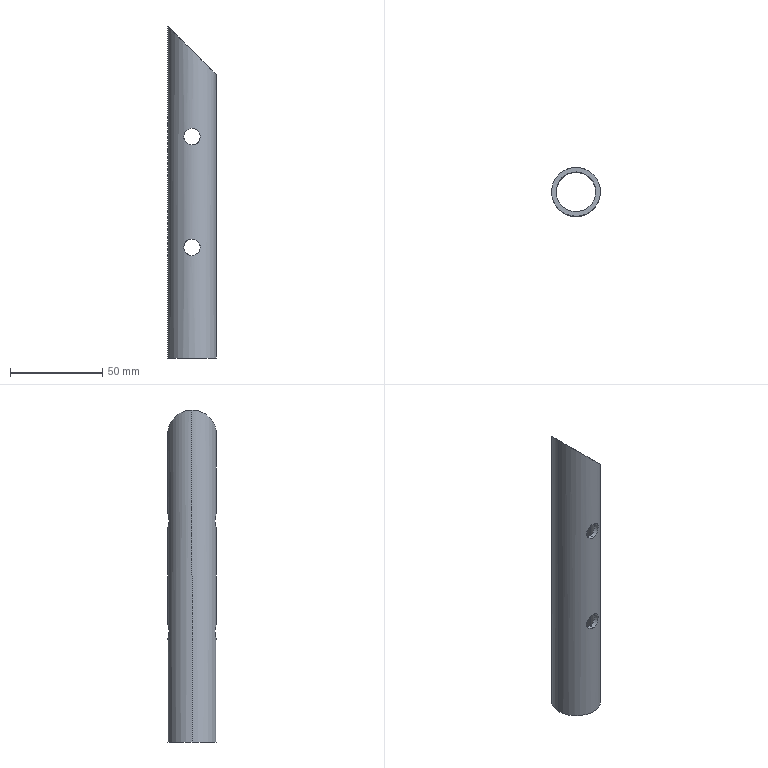Part | NX | features BREP 1 | 1 solid | 14 faces | box 26.5 x 26.5 x 180 mm | volume 30784 mm3 | cylinder 12 | plane 2 | commonest cylinder face diameters 9 x8 21.5 x2 26.5 x2
STEP:
#1=CARTESIAN_POINT('',(0.,10.75,25.5));
#2=VERTEX_POINT('',#1);
#3=CARTESIAN_POINT('',(0.,10.75,34.5));
#4=VERTEX_POINT('',#3);
#5=CARTESIAN_POINT('',(0.,10.75,25.5));
#6=CARTESIAN_POINT('',(1.204,10.75,25.5));
#7=CARTESIAN_POINT('',(3.514,10.279,26.479));
#8=CARTESIAN_POINT('',(4.992,9.505,29.99));
#9=CARTESIAN_POINT('',(3.516,10.279,33.525));
#10=CARTESIAN_POINT('',(1.204,10.75,34.5));
#11=CARTESIAN_POINT('',(0.,10.75,34.5));
#12=B_SPLINE_CURVE_WITH_KNOTS('',3,(#5,#6,#7,#8,#9,#10,#11),.UNSPECIFIED.,.F.,.F.,(4,1,1,1,4),(0.,0.003557,0.007114,0.01067,0.01423),.UNSPECIFIED.);
#13=EDGE_CURVE('',#2,#4,#12,.T.);
#14=ORIENTED_EDGE('',*,*,#13,.T.);
#15=CARTESIAN_POINT('',(0.,13.25,34.5));
#16=VERTEX_POINT('',#15);
#17=CARTESIAN_POINT('',(0.,13.25,34.5));
#18=DIRECTION('',(0.,-1.,0.));
#19=VECTOR('',#18,1000.);
#20=LINE('',#17,#19);
#21=EDGE_CURVE('',#16,#4,#20,.T.);
#22=ORIENTED_EDGE('',*,*,#21,.F.);
#23=CARTESIAN_POINT('',(0.,13.25,25.5));
#24=VERTEX_POINT('',#23);
#25=CARTESIAN_POINT('',(0.,13.25,34.5));
#26=CARTESIAN_POINT('',(1.198,13.25,34.5));
#27=CARTESIAN_POINT('',(3.516,12.868,33.523));
#28=CARTESIAN_POINT('',(4.992,12.26,30.008));
#29=CARTESIAN_POINT('',(3.518,12.867,26.474));
#30=CARTESIAN_POINT('',(1.199,13.25,25.5));
#31=CARTESIAN_POINT('',(0.,13.25,25.5));
#32=B_SPLINE_CURVE_WITH_KNOTS('',3,(#25,#26,#27,#28,#29,#30,#31),.UNSPECIFIED.,.F.,.F.,(4,1,1,1,4),(0.,0.003542,0.007085,0.01063,0.01417),.UNSPECIFIED.);
#33=EDGE_CURVE('',#16,#24,#32,.T.);
#34=ORIENTED_EDGE('',*,*,#33,.T.);
#35=CARTESIAN_POINT('',(0.,13.25,25.5));
#36=DIRECTION('',(0.,-1.,0.));
#37=VECTOR('',#36,1000.);
#38=LINE('',#35,#37);
#39=EDGE_CURVE('',#24,#2,#38,.T.);
#40=ORIENTED_EDGE('',*,*,#39,.T.);
#41=EDGE_LOOP('',(#14,#22,#34,#40));
#42=FACE_BOUND('',#41,.T.);
#43=CARTESIAN_POINT('',(0.,-100.,30.));
#44=DIRECTION('',(0.,1.,0.));
#45=DIRECTION('',(0.,0.,-1.));
#46=AXIS2_PLACEMENT_3D('',#43,#44,#45);
#47=CYLINDRICAL_SURFACE('',#46,4.5);
#48=ADVANCED_FACE('',(#42),#47,.F.);
#49=ORIENTED_EDGE('',*,*,#39,.F.);
#50=CARTESIAN_POINT('',(0.,13.25,25.5));
#51=CARTESIAN_POINT('',(-1.198,13.25,25.5));
#52=CARTESIAN_POINT('',(-3.516,12.868,26.477));
#53=CARTESIAN_POINT('',(-4.992,12.26,29.992));
#54=CARTESIAN_POINT('',(-3.518,12.867,33.526));
#55=CARTESIAN_POINT('',(-1.199,13.25,34.5));
#56=CARTESIAN_POINT('',(0.,13.25,34.5));
#57=B_SPLINE_CURVE_WITH_KNOTS('',3,(#50,#51,#52,#53,#54,#55,#56),.UNSPECIFIED.,.F.,.F.,(4,1,1,1,4),(0.,0.003542,0.007085,0.01063,0.01417),.UNSPECIFIED.);
#58=EDGE_CURVE('',#24,#16,#57,.T.);
#59=ORIENTED_EDGE('',*,*,#58,.T.);
#60=ORIENTED_EDGE('',*,*,#21,.T.);
#61=CARTESIAN_POINT('',(0.,10.75,25.5));
#62=CARTESIAN_POINT('',(-1.204,10.75,25.5));
#63=CARTESIAN_POINT('',(-3.514,10.279,26.479));
#64=CARTESIAN_POINT('',(-4.992,9.505,29.99));
#65=CARTESIAN_POINT('',(-3.516,10.279,33.525));
#66=CARTESIAN_POINT('',(-1.204,10.75,34.5));
#67=CARTESIAN_POINT('',(0.,10.75,34.5));
#68=B_SPLINE_CURVE_WITH_KNOTS('',3,(#61,#62,#63,#64,#65,#66,#67),.UNSPECIFIED.,.F.,.F.,(4,1,1,1,4),(0.,0.003557,0.007114,0.01067,0.01423),.UNSPECIFIED.);
#69=EDGE_CURVE('',#2,#4,#68,.T.);
#70=ORIENTED_EDGE('',*,*,#69,.F.);
#71=EDGE_LOOP('',(#49,#59,#60,#70));
#72=FACE_BOUND('',#71,.T.);
#73=CARTESIAN_POINT('',(0.,-100.,30.));
#74=DIRECTION('',(0.,1.,0.));
#75=DIRECTION('',(0.,0.,-1.));
#76=AXIS2_PLACEMENT_3D('',#73,#74,#75);
#77=CYLINDRICAL_SURFACE('',#76,4.5);
#78=ADVANCED_FACE('',(#72),#77,.F.);
#79=CARTESIAN_POINT('',(10.75,0.,66.));
#80=VERTEX_POINT('',#79);
#81=CARTESIAN_POINT('',(-10.75,0.,87.5));
#82=VERTEX_POINT('',#81);
#83=CARTESIAN_POINT('',(0.,0.,76.75));
#84=DIRECTION('',(-0.7071,0.,-0.7071));
#85=DIRECTION('',(0.7071,0.,-0.7071));
#86=AXIS2_PLACEMENT_3D('',#83,#84,#85);
#87=ELLIPSE('',#86,15.203,10.75);
#88=EDGE_CURVE('',#80,#82,#87,.F.);
#89=ORIENTED_EDGE('',*,*,#88,.T.);
#90=CARTESIAN_POINT('',(-10.75,0.,-90.));
#91=VERTEX_POINT('',#90);
#92=CARTESIAN_POINT('',(-10.75,0.,-90.));
#93=DIRECTION('',(0.,0.,1.));
#94=VECTOR('',#93,1000.);
#95=LINE('',#92,#94);
#96=EDGE_CURVE('',#82,#91,#95,.F.);
#97=ORIENTED_EDGE('',*,*,#96,.T.);
#98=CARTESIAN_POINT('',(10.75,0.,-90.));
#99=VERTEX_POINT('',#98);
#100=CARTESIAN_POINT('',(0.,0.,-90.));
#101=DIRECTION('',(0.,0.,1.));
#102=DIRECTION('',(1.,0.,0.));
#103=AXIS2_PLACEMENT_3D('',#100,#101,#102);
#104=CIRCLE('',#103,10.75);
#105=EDGE_CURVE('',#99,#91,#104,.T.);
#106=ORIENTED_EDGE('',*,*,#105,.F.);
#107=CARTESIAN_POINT('',(10.75,0.,-90.));
#108=DIRECTION('',(0.,0.,1.));
#109=VECTOR('',#108,1000.);
#110=LINE('',#107,#109);
#111=EDGE_CURVE('',#80,#99,#110,.F.);
#112=ORIENTED_EDGE('',*,*,#111,.F.);
#113=EDGE_LOOP('',(#89,#97,#106,#112));
#114=FACE_BOUND('',#113,.T.);
#115=ORIENTED_EDGE('',*,*,#13,.F.);
#116=ORIENTED_EDGE('',*,*,#69,.T.);
#117=EDGE_LOOP('',(#115,#116));
#118=FACE_BOUND('',#117,.T.);
#119=CARTESIAN_POINT('',(0.,10.75,-34.5));
#120=VERTEX_POINT('',#119);
#121=CARTESIAN_POINT('',(0.,10.75,-25.5));
#122=VERTEX_POINT('',#121);
#123=CARTESIAN_POINT('',(0.,10.75,-34.5));
#124=CARTESIAN_POINT('',(1.204,10.75,-34.5));
#125=CARTESIAN_POINT('',(3.514,10.279,-33.521));
#126=CARTESIAN_POINT('',(4.992,9.505,-30.01));
#127=CARTESIAN_POINT('',(3.516,10.279,-26.475));
#128=CARTESIAN_POINT('',(1.204,10.75,-25.5));
#129=CARTESIAN_POINT('',(0.,10.75,-25.5));
#130=B_SPLINE_CURVE_WITH_KNOTS('',3,(#123,#124,#125,#126,#127,#128,#129),.UNSPECIFIED.,.F.,.F.,(4,1,1,1,4),(0.,0.003557,0.007114,0.01067,0.01423),.UNSPECIFIED.);
#131=EDGE_CURVE('',#120,#122,#130,.T.);
#132=ORIENTED_EDGE('',*,*,#131,.F.);
#133=CARTESIAN_POINT('',(0.,10.75,-34.5));
#134=CARTESIAN_POINT('',(-1.204,10.75,-34.5));
#135=CARTESIAN_POINT('',(-3.514,10.279,-33.521));
#136=CARTESIAN_POINT('',(-4.992,9.505,-30.01));
#137=CARTESIAN_POINT('',(-3.516,10.279,-26.475));
#138=CARTESIAN_POINT('',(-1.204,10.75,-25.5));
#139=CARTESIAN_POINT('',(0.,10.75,-25.5));
#140=B_SPLINE_CURVE_WITH_KNOTS('',3,(#133,#134,#135,#136,#137,#138,#139),.UNSPECIFIED.,.F.,.F.,(4,1,1,1,4),(0.,0.003557,0.007114,0.01067,0.01423),.UNSPECIFIED.);
#141=EDGE_CURVE('',#120,#122,#140,.T.);
#142=ORIENTED_EDGE('',*,*,#141,.T.);
#143=EDGE_LOOP('',(#132,#142));
#144=FACE_BOUND('',#143,.T.);
#145=CARTESIAN_POINT('',(0.,0.,90.));
#146=DIRECTION('',(0.,0.,-1.));
#147=DIRECTION('',(1.,0.,0.));
#148=AXIS2_PLACEMENT_3D('',#145,#146,#147);
#149=CYLINDRICAL_SURFACE('',#148,10.75);
#150=ADVANCED_FACE('',(#114,#118,#144),#149,.F.);
#151=ORIENTED_EDGE('',*,*,#111,.T.);
#152=CARTESIAN_POINT('',(0.,0.,-90.));
#153=DIRECTION('',(0.,0.,1.));
#154=DIRECTION('',(-1.,0.,0.));
#155=AXIS2_PLACEMENT_3D('',#152,#153,#154);
#156=CIRCLE('',#155,10.75);
#157=EDGE_CURVE('',#91,#99,#156,.T.);
#158=ORIENTED_EDGE('',*,*,#157,.F.);
#159=ORIENTED_EDGE('',*,*,#96,.F.);
#160=CARTESIAN_POINT('',(0.,0.,76.75));
#161=DIRECTION('',(-0.7071,0.,-0.7071));
#162=DIRECTION('',(0.7071,0.,-0.7071));
#163=AXIS2_PLACEMENT_3D('',#160,#161,#162);
#164=ELLIPSE('',#163,15.203,10.75);
#165=EDGE_CURVE('',#82,#80,#164,.F.);
#166=ORIENTED_EDGE('',*,*,#165,.T.);
#167=EDGE_LOOP('',(#151,#158,#159,#166));
#168=FACE_BOUND('',#167,.T.);
#169=CARTESIAN_POINT('',(0.,-10.75,-34.5));
#170=VERTEX_POINT('',#169);
#171=CARTESIAN_POINT('',(0.,-10.75,-25.5));
#172=VERTEX_POINT('',#171);
#173=CARTESIAN_POINT('',(0.,-10.75,-34.5));
#174=CARTESIAN_POINT('',(-1.204,-10.75,-34.5));
#175=CARTESIAN_POINT('',(-3.514,-10.279,-33.521));
#176=CARTESIAN_POINT('',(-4.992,-9.505,-30.01));
#177=CARTESIAN_POINT('',(-3.516,-10.279,-26.475));
#178=CARTESIAN_POINT('',(-1.204,-10.75,-25.5));
#179=CARTESIAN_POINT('',(0.,-10.75,-25.5));
#180=B_SPLINE_CURVE_WITH_KNOTS('',3,(#173,#174,#175,#176,#177,#178,#179),.UNSPECIFIED.,.F.,.F.,(4,1,1,1,4),(0.,0.003557,0.007114,0.01067,0.01423),.UNSPECIFIED.);
#181=EDGE_CURVE('',#170,#172,#180,.T.);
#182=ORIENTED_EDGE('',*,*,#181,.F.);
#183=CARTESIAN_POINT('',(0.,-10.75,-34.5));
#184=CARTESIAN_POINT('',(1.204,-10.75,-34.5));
#185=CARTESIAN_POINT('',(3.514,-10.279,-33.521));
#186=CARTESIAN_POINT('',(4.992,-9.505,-30.01));
#187=CARTESIAN_POINT('',(3.516,-10.279,-26.475));
#188=CARTESIAN_POINT('',(1.204,-10.75,-25.5));
#189=CARTESIAN_POINT('',(0.,-10.75,-25.5));
#190=B_SPLINE_CURVE_WITH_KNOTS('',3,(#183,#184,#185,#186,#187,#188,#189),.UNSPECIFIED.,.F.,.F.,(4,1,1,1,4),(0.,0.003557,0.007114,0.01067,0.01423),.UNSPECIFIED.);
#191=EDGE_CURVE('',#170,#172,#190,.T.);
#192=ORIENTED_EDGE('',*,*,#191,.T.);
#193=EDGE_LOOP('',(#182,#192));
#194=FACE_BOUND('',#193,.T.);
#195=CARTESIAN_POINT('',(0.,-10.75,25.5));
#196=VERTEX_POINT('',#195);
#197=CARTESIAN_POINT('',(0.,-10.75,34.5));
#198=VERTEX_POINT('',#197);
#199=CARTESIAN_POINT('',(0.,-10.75,25.5));
#200=CARTESIAN_POINT('',(-1.204,-10.75,25.5));
#201=CARTESIAN_POINT('',(-3.514,-10.279,26.479));
#202=CARTESIAN_POINT('',(-4.992,-9.505,29.99));
#203=CARTESIAN_POINT('',(-3.516,-10.279,33.525));
#204=CARTESIAN_POINT('',(-1.204,-10.75,34.5));
#205=CARTESIAN_POINT('',(0.,-10.75,34.5));
#206=B_SPLINE_CURVE_WITH_KNOTS('',3,(#199,#200,#201,#202,#203,#204,#205),.UNSPECIFIED.,.F.,.F.,(4,1,1,1,4),(0.,0.003557,0.007114,0.01067,0.01423),.UNSPECIFIED.);
#207=EDGE_CURVE('',#196,#198,#206,.T.);
#208=ORIENTED_EDGE('',*,*,#207,.F.);
#209=CARTESIAN_POINT('',(0.,-10.75,25.5));
#210=CARTESIAN_POINT('',(1.204,-10.75,25.5));
#211=CARTESIAN_POINT('',(3.514,-10.279,26.479));
#212=CARTESIAN_POINT('',(4.992,-9.505,29.99));
#213=CARTESIAN_POINT('',(3.516,-10.279,33.525));
#214=CARTESIAN_POINT('',(1.204,-10.75,34.5));
#215=CARTESIAN_POINT('',(0.,-10.75,34.5));
#216=B_SPLINE_CURVE_WITH_KNOTS('',3,(#209,#210,#211,#212,#213,#214,#215),.UNSPECIFIED.,.F.,.F.,(4,1,1,1,4),(0.,0.003557,0.007114,0.01067,0.01423),.UNSPECIFIED.);
#217=EDGE_CURVE('',#196,#198,#216,.T.);
#218=ORIENTED_EDGE('',*,*,#217,.T.);
#219=EDGE_LOOP('',(#208,#218));
#220=FACE_BOUND('',#219,.T.);
#221=CARTESIAN_POINT('',(0.,0.,90.));
#222=DIRECTION('',(0.,0.,-1.));
#223=DIRECTION('',(1.,0.,0.));
#224=AXIS2_PLACEMENT_3D('',#221,#222,#223);
#225=CYLINDRICAL_SURFACE('',#224,10.75);
#226=ADVANCED_FACE('',(#168,#194,#220),#225,.F.);
#227=CARTESIAN_POINT('',(-13.25,0.,90.));
#228=VERTEX_POINT('',#227);
#229=CARTESIAN_POINT('',(13.25,0.,63.5));
#230=VERTEX_POINT('',#229);
#231=CARTESIAN_POINT('',(0.,0.,76.75));
#232=DIRECTION('',(-0.7071,0.,-0.7071));
#233=DIRECTION('',(0.7071,0.,-0.7071));
#234=AXIS2_PLACEMENT_3D('',#231,#232,#233);
#235=ELLIPSE('',#234,18.738,13.25);
#236=EDGE_CURVE('',#228,#230,#235,.F.);
#237=ORIENTED_EDGE('',*,*,#236,.T.);
#238=CARTESIAN_POINT('',(0.,0.,76.75));
#239=DIRECTION('',(-0.7071,0.,-0.7071));
#240=DIRECTION('',(0.7071,0.,-0.7071));
#241=AXIS2_PLACEMENT_3D('',#238,#239,#240);
#242=ELLIPSE('',#241,18.738,13.25);
#243=EDGE_CURVE('',#230,#228,#242,.F.);
#244=ORIENTED_EDGE('',*,*,#243,.T.);
#245=EDGE_LOOP('',(#237,#244));
#246=FACE_BOUND('',#245,.T.);
#247=ORIENTED_EDGE('',*,*,#165,.F.);
#248=ORIENTED_EDGE('',*,*,#88,.F.);
#249=EDGE_LOOP('',(#247,#248));
#250=FACE_BOUND('',#249,.T.);
#251=CARTESIAN_POINT('',(-13.25,-100.,90.));
#252=DIRECTION('',(-0.7071,0.,-0.7071));
#253=DIRECTION('',(0.7071,0.,-0.7071));
#254=AXIS2_PLACEMENT_3D('',#251,#252,#253);
#255=PLANE('',#254);
#256=ADVANCED_FACE('',(#246,#250),#255,.F.);
#257=CARTESIAN_POINT('',(13.25,0.,-90.));
#258=VERTEX_POINT('',#257);
#259=CARTESIAN_POINT('',(13.25,0.,-90.));
#260=DIRECTION('',(0.,0.,1.));
#261=VECTOR('',#260,1000.);
#262=LINE('',#259,#261);
#263=EDGE_CURVE('',#258,#230,#262,.T.);
#264=ORIENTED_EDGE('',*,*,#263,.F.);
#265=CARTESIAN_POINT('',(-13.25,0.,-90.));
#266=VERTEX_POINT('',#265);
#267=CARTESIAN_POINT('',(0.,0.,-90.));
#268=DIRECTION('',(0.,0.,-1.));
#269=DIRECTION('',(-1.,0.,0.));
#270=AXIS2_PLACEMENT_3D('',#267,#268,#269);
#271=CIRCLE('',#270,13.25);
#272=EDGE_CURVE('',#266,#258,#271,.T.);
#273=ORIENTED_EDGE('',*,*,#272,.F.);
#274=CARTESIAN_POINT('',(-13.25,0.,-90.));
#275=DIRECTION('',(0.,0.,1.));
#276=VECTOR('',#275,1000.);
#277=LINE('',#274,#276);
#278=EDGE_CURVE('',#266,#228,#277,.T.);
#279=ORIENTED_EDGE('',*,*,#278,.T.);
#280=ORIENTED_EDGE('',*,*,#243,.F.);
#281=EDGE_LOOP('',(#264,#273,#279,#280));
#282=FACE_BOUND('',#281,.T.);
#283=CARTESIAN_POINT('',(0.,13.25,-25.5));
#284=VERTEX_POINT('',#283);
#285=CARTESIAN_POINT('',(0.,13.25,-34.5));
#286=VERTEX_POINT('',#285);
#287=CARTESIAN_POINT('',(0.,13.25,-25.5));
#288=CARTESIAN_POINT('',(1.198,13.25,-25.5));
#289=CARTESIAN_POINT('',(3.516,12.868,-26.477));
#290=CARTESIAN_POINT('',(4.992,12.26,-29.992));
#291=CARTESIAN_POINT('',(3.518,12.867,-33.526));
#292=CARTESIAN_POINT('',(1.199,13.25,-34.5));
#293=CARTESIAN_POINT('',(0.,13.25,-34.5));
#294=B_SPLINE_CURVE_WITH_KNOTS('',3,(#287,#288,#289,#290,#291,#292,#293),.UNSPECIFIED.,.F.,.F.,(4,1,1,1,4),(0.,0.003542,0.007085,0.01063,0.01417),.UNSPECIFIED.);
#295=EDGE_CURVE('',#284,#286,#294,.T.);
#296=ORIENTED_EDGE('',*,*,#295,.F.);
#297=CARTESIAN_POINT('',(0.,13.25,-34.5));
#298=CARTESIAN_POINT('',(-1.198,13.25,-34.5));
#299=CARTESIAN_POINT('',(-3.516,12.868,-33.523));
#300=CARTESIAN_POINT('',(-4.992,12.26,-30.008));
#301=CARTESIAN_POINT('',(-3.518,12.867,-26.474));
#302=CARTESIAN_POINT('',(-1.199,13.25,-25.5));
#303=CARTESIAN_POINT('',(0.,13.25,-25.5));
#304=B_SPLINE_CURVE_WITH_KNOTS('',3,(#297,#298,#299,#300,#301,#302,#303),.UNSPECIFIED.,.F.,.F.,(4,1,1,1,4),(0.,0.003542,0.007085,0.01063,0.01417),.UNSPECIFIED.);
#305=EDGE_CURVE('',#286,#284,#304,.T.);
#306=ORIENTED_EDGE('',*,*,#305,.F.);
#307=EDGE_LOOP('',(#296,#306));
#308=FACE_BOUND('',#307,.T.);
#309=ORIENTED_EDGE('',*,*,#33,.F.);
#310=ORIENTED_EDGE('',*,*,#58,.F.);
#311=EDGE_LOOP('',(#309,#310));
#312=FACE_BOUND('',#311,.T.);
#313=CARTESIAN_POINT('',(0.,0.,90.));
#314=DIRECTION('',(0.,0.,-1.));
#315=DIRECTION('',(1.,0.,0.));
#316=AXIS2_PLACEMENT_3D('',#313,#314,#315);
#317=CYLINDRICAL_SURFACE('',#316,13.25);
#318=ADVANCED_FACE('',(#282,#308,#312),#317,.T.);
#319=ORIENTED_EDGE('',*,*,#236,.F.);
#320=ORIENTED_EDGE('',*,*,#278,.F.);
#321=CARTESIAN_POINT('',(0.,0.,-90.));
#322=DIRECTION('',(0.,0.,-1.));
#323=DIRECTION('',(1.,0.,0.));
#324=AXIS2_PLACEMENT_3D('',#321,#322,#323);
#325=CIRCLE('',#324,13.25);
#326=EDGE_CURVE('',#258,#266,#325,.T.);
#327=ORIENTED_EDGE('',*,*,#326,.F.);
#328=ORIENTED_EDGE('',*,*,#263,.T.);
#329=EDGE_LOOP('',(#319,#320,#327,#328));
#330=FACE_BOUND('',#329,.T.);
#331=CARTESIAN_POINT('',(0.,-13.25,34.5));
#332=VERTEX_POINT('',#331);
#333=CARTESIAN_POINT('',(0.,-13.25,25.5));
#334=VERTEX_POINT('',#333);
#335=CARTESIAN_POINT('',(0.,-13.25,34.5));
#336=CARTESIAN_POINT('',(-1.198,-13.25,34.5));
#337=CARTESIAN_POINT('',(-3.516,-12.868,33.523));
#338=CARTESIAN_POINT('',(-4.992,-12.26,30.008));
#339=CARTESIAN_POINT('',(-3.518,-12.867,26.474));
#340=CARTESIAN_POINT('',(-1.199,-13.25,25.5));
#341=CARTESIAN_POINT('',(0.,-13.25,25.5));
#342=B_SPLINE_CURVE_WITH_KNOTS('',3,(#335,#336,#337,#338,#339,#340,#341),.UNSPECIFIED.,.F.,.F.,(4,1,1,1,4),(0.,0.003542,0.007085,0.01063,0.01417),.UNSPECIFIED.);
#343=EDGE_CURVE('',#332,#334,#342,.T.);
#344=ORIENTED_EDGE('',*,*,#343,.F.);
#345=CARTESIAN_POINT('',(0.,-13.25,25.5));
#346=CARTESIAN_POINT('',(1.198,-13.25,25.5));
#347=CARTESIAN_POINT('',(3.516,-12.868,26.477));
#348=CARTESIAN_POINT('',(4.992,-12.26,29.992));
#349=CARTESIAN_POINT('',(3.518,-12.867,33.526));
#350=CARTESIAN_POINT('',(1.199,-13.25,34.5));
#351=CARTESIAN_POINT('',(0.,-13.25,34.5));
#352=B_SPLINE_CURVE_WITH_KNOTS('',3,(#345,#346,#347,#348,#349,#350,#351),.UNSPECIFIED.,.F.,.F.,(4,1,1,1,4),(0.,0.003542,0.007085,0.01063,0.01417),.UNSPECIFIED.);
#353=EDGE_CURVE('',#334,#332,#352,.T.);
#354=ORIENTED_EDGE('',*,*,#353,.F.);
#355=EDGE_LOOP('',(#344,#354));
#356=FACE_BOUND('',#355,.T.);
#357=CARTESIAN_POINT('',(0.,-13.25,-25.5));
#358=VERTEX_POINT('',#357);
#359=CARTESIAN_POINT('',(0.,-13.25,-34.5));
#360=VERTEX_POINT('',#359);
#361=CARTESIAN_POINT('',(0.,-13.25,-25.5));
#362=CARTESIAN_POINT('',(-1.198,-13.25,-25.5));
#363=CARTESIAN_POINT('',(-3.516,-12.868,-26.477));
#364=CARTESIAN_POINT('',(-4.992,-12.26,-29.992));
#365=CARTESIAN_POINT('',(-3.518,-12.867,-33.526));
#366=CARTESIAN_POINT('',(-1.199,-13.25,-34.5));
#367=CARTESIAN_POINT('',(0.,-13.25,-34.5));
#368=B_SPLINE_CURVE_WITH_KNOTS('',3,(#361,#362,#363,#364,#365,#366,#367),.UNSPECIFIED.,.F.,.F.,(4,1,1,1,4),(0.,0.003542,0.007085,0.01063,0.01417),.UNSPECIFIED.);
#369=EDGE_CURVE('',#358,#360,#368,.T.);
#370=ORIENTED_EDGE('',*,*,#369,.F.);
#371=CARTESIAN_POINT('',(0.,-13.25,-34.5));
#372=CARTESIAN_POINT('',(1.198,-13.25,-34.5));
#373=CARTESIAN_POINT('',(3.516,-12.868,-33.523));
#374=CARTESIAN_POINT('',(4.992,-12.26,-30.008));
#375=CARTESIAN_POINT('',(3.518,-12.867,-26.474));
#376=CARTESIAN_POINT('',(1.199,-13.25,-25.5));
#377=CARTESIAN_POINT('',(0.,-13.25,-25.5));
#378=B_SPLINE_CURVE_WITH_KNOTS('',3,(#371,#372,#373,#374,#375,#376,#377),.UNSPECIFIED.,.F.,.F.,(4,1,1,1,4),(0.,0.003542,0.007085,0.01063,0.01417),.UNSPECIFIED.);
#379=EDGE_CURVE('',#360,#358,#378,.T.);
#380=ORIENTED_EDGE('',*,*,#379,.F.);
#381=EDGE_LOOP('',(#370,#380));
#382=FACE_BOUND('',#381,.T.);
#383=CARTESIAN_POINT('',(0.,0.,90.));
#384=DIRECTION('',(0.,0.,-1.));
#385=DIRECTION('',(1.,0.,0.));
#386=AXIS2_PLACEMENT_3D('',#383,#384,#385);
#387=CYLINDRICAL_SURFACE('',#386,13.25);
#388=ADVANCED_FACE('',(#330,#356,#382),#387,.T.);
#389=ORIENTED_EDGE('',*,*,#272,.T.);
#390=ORIENTED_EDGE('',*,*,#326,.T.);
#391=EDGE_LOOP('',(#389,#390));
#392=FACE_BOUND('',#391,.T.);
#393=ORIENTED_EDGE('',*,*,#105,.T.);
#394=ORIENTED_EDGE('',*,*,#157,.T.);
#395=EDGE_LOOP('',(#393,#394));
#396=FACE_BOUND('',#395,.T.);
#397=CARTESIAN_POINT('',(0.,0.,-90.));
#398=DIRECTION('',(0.,0.,1.));
#399=DIRECTION('',(-1.,0.,0.));
#400=AXIS2_PLACEMENT_3D('',#397,#398,#399);
#401=PLANE('',#400);
#402=ADVANCED_FACE('',(#392,#396),#401,.F.);
#403=ORIENTED_EDGE('',*,*,#353,.T.);
#404=CARTESIAN_POINT('',(0.,-10.75,34.5));
#405=DIRECTION('',(0.,-1.,0.));
#406=VECTOR('',#405,1000.);
#407=LINE('',#404,#406);
#408=EDGE_CURVE('',#198,#332,#407,.T.);
#409=ORIENTED_EDGE('',*,*,#408,.F.);
#410=ORIENTED_EDGE('',*,*,#217,.F.);
#411=CARTESIAN_POINT('',(0.,-10.75,25.5));
#412=DIRECTION('',(0.,-1.,0.));
#413=VECTOR('',#412,1000.);
#414=LINE('',#411,#413);
#415=EDGE_CURVE('',#196,#334,#414,.T.);
#416=ORIENTED_EDGE('',*,*,#415,.T.);
#417=EDGE_LOOP('',(#403,#409,#410,#416));
#418=FACE_BOUND('',#417,.T.);
#419=CARTESIAN_POINT('',(0.,-100.,30.));
#420=DIRECTION('',(0.,1.,0.));
#421=DIRECTION('',(0.,0.,-1.));
#422=AXIS2_PLACEMENT_3D('',#419,#420,#421);
#423=CYLINDRICAL_SURFACE('',#422,4.5);
#424=ADVANCED_FACE('',(#418),#423,.F.);
#425=ORIENTED_EDGE('',*,*,#415,.F.);
#426=ORIENTED_EDGE('',*,*,#207,.T.);
#427=ORIENTED_EDGE('',*,*,#408,.T.);
#428=ORIENTED_EDGE('',*,*,#343,.T.);
#429=EDGE_LOOP('',(#425,#426,#427,#428));
#430=FACE_BOUND('',#429,.T.);
#431=CARTESIAN_POINT('',(0.,-100.,30.));
#432=DIRECTION('',(0.,1.,0.));
#433=DIRECTION('',(0.,0.,-1.));
#434=AXIS2_PLACEMENT_3D('',#431,#432,#433);
#435=CYLINDRICAL_SURFACE('',#434,4.5);
#436=ADVANCED_FACE('',(#430),#435,.F.);
#437=ORIENTED_EDGE('',*,*,#379,.T.);
#438=CARTESIAN_POINT('',(0.,-10.75,-25.5));
#439=DIRECTION('',(0.,-1.,0.));
#440=VECTOR('',#439,1000.);
#441=LINE('',#438,#440);
#442=EDGE_CURVE('',#172,#358,#441,.T.);
#443=ORIENTED_EDGE('',*,*,#442,.F.);
#444=ORIENTED_EDGE('',*,*,#191,.F.);
#445=CARTESIAN_POINT('',(0.,-10.75,-34.5));
#446=DIRECTION('',(0.,-1.,0.));
#447=VECTOR('',#446,1000.);
#448=LINE('',#445,#447);
#449=EDGE_CURVE('',#170,#360,#448,.T.);
#450=ORIENTED_EDGE('',*,*,#449,.T.);
#451=EDGE_LOOP('',(#437,#443,#444,#450));
#452=FACE_BOUND('',#451,.T.);
#453=CARTESIAN_POINT('',(0.,-100.,-30.));
#454=DIRECTION('',(0.,1.,0.));
#455=DIRECTION('',(0.,0.,-1.));
#456=AXIS2_PLACEMENT_3D('',#453,#454,#455);
#457=CYLINDRICAL_SURFACE('',#456,4.5);
#458=ADVANCED_FACE('',(#452),#457,.F.);
#459=ORIENTED_EDGE('',*,*,#449,.F.);
#460=ORIENTED_EDGE('',*,*,#181,.T.);
#461=ORIENTED_EDGE('',*,*,#442,.T.);
#462=ORIENTED_EDGE('',*,*,#369,.T.);
#463=EDGE_LOOP('',(#459,#460,#461,#462));
#464=FACE_BOUND('',#463,.T.);
#465=CARTESIAN_POINT('',(0.,-100.,-30.));
#466=DIRECTION('',(0.,1.,0.));
#467=DIRECTION('',(0.,0.,-1.));
#468=AXIS2_PLACEMENT_3D('',#465,#466,#467);
#469=CYLINDRICAL_SURFACE('',#468,4.5);
#470=ADVANCED_FACE('',(#464),#469,.F.);
#471=CARTESIAN_POINT('',(0.,13.25,-34.5));
#472=DIRECTION('',(0.,-1.,0.));
#473=VECTOR('',#472,1000.);
#474=LINE('',#471,#473);
#475=EDGE_CURVE('',#120,#286,#474,.F.);
#476=ORIENTED_EDGE('',*,*,#475,.T.);
#477=ORIENTED_EDGE('',*,*,#305,.T.);
#478=CARTESIAN_POINT('',(0.,13.25,-25.5));
#479=DIRECTION('',(0.,-1.,0.));
#480=VECTOR('',#479,1000.);
#481=LINE('',#478,#480);
#482=EDGE_CURVE('',#122,#284,#481,.F.);
#483=ORIENTED_EDGE('',*,*,#482,.F.);
#484=ORIENTED_EDGE('',*,*,#141,.F.);
#485=EDGE_LOOP('',(#476,#477,#483,#484));
#486=FACE_BOUND('',#485,.T.);
#487=CARTESIAN_POINT('',(0.,-100.,-30.));
#488=DIRECTION('',(0.,1.,0.));
#489=DIRECTION('',(0.,0.,-1.));
#490=AXIS2_PLACEMENT_3D('',#487,#488,#489);
#491=CYLINDRICAL_SURFACE('',#490,4.5);
#492=ADVANCED_FACE('',(#486),#491,.F.);
#493=ORIENTED_EDGE('',*,*,#131,.T.);
#494=ORIENTED_EDGE('',*,*,#482,.T.);
#495=ORIENTED_EDGE('',*,*,#295,.T.);
#496=ORIENTED_EDGE('',*,*,#475,.F.);
#497=EDGE_LOOP('',(#493,#494,#495,#496));
#498=FACE_BOUND('',#497,.T.);
#499=CARTESIAN_POINT('',(0.,-100.,-30.));
#500=DIRECTION('',(0.,1.,0.));
#501=DIRECTION('',(0.,0.,-1.));
#502=AXIS2_PLACEMENT_3D('',#499,#500,#501);
#503=CYLINDRICAL_SURFACE('',#502,4.5);
#504=ADVANCED_FACE('',(#498),#503,.F.);
#505=CLOSED_SHELL('',(#48,#78,#150,#226,#256,#318,#388,#402,#424,#436,#458,#470,#492,#504));
#506=MANIFOLD_SOLID_BREP('',#505);
#507=(LENGTH_UNIT()NAMED_UNIT(*)SI_UNIT(.MILLI.,.METRE.));
#508=UNCERTAINTY_MEASURE_WITH_UNIT(LENGTH_MEASURE(0.0508),#507,'','');
#509=(NAMED_UNIT(*)PLANE_ANGLE_UNIT()SI_UNIT($,.RADIAN.));
#510=(NAMED_UNIT(*)SI_UNIT($,.STERADIAN.)SOLID_ANGLE_UNIT());
#511=(GEOMETRIC_REPRESENTATION_CONTEXT(3)GLOBAL_UNCERTAINTY_ASSIGNED_CONTEXT((#508))GLOBAL_UNIT_ASSIGNED_CONTEXT((#507,#509,#510))REPRESENTATION_CONTEXT('',''));
#512=ADVANCED_BREP_SHAPE_REPRESENTATION('',(#506),#511);